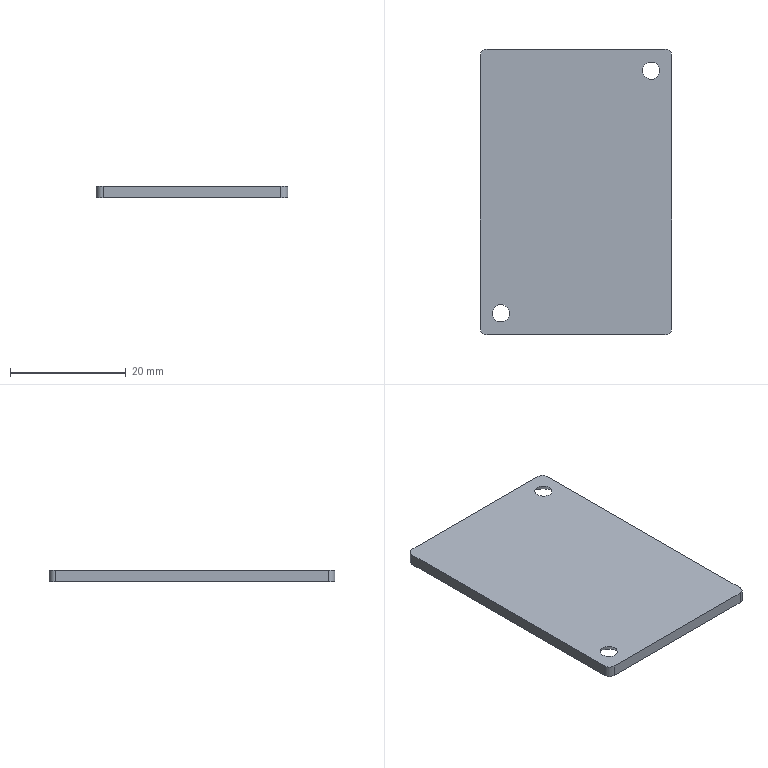Part | STEP file | 4V430C_15_Valve_Board | 1 solid | 14 faces | box 33.2 x 49.5 x 2 mm | volume 3202 mm3 | plane 6 | cone 4 | cylinder 4 | commonest cylinder face diameters 2.4 x4
STEP:
#1=CARTESIAN_POINT('',(0.,0.,0.));
#2=DIRECTION('',(0.,0.,1.));
#3=DIRECTION('',(1.,0.,0.));
#4=AXIS2_PLACEMENT_3D('',#1,#2,#3);
#5=CARTESIAN_POINT('',(-14.5,-21.,0.));
#6=VERTEX_POINT('',#5);
#7=CARTESIAN_POINT('',(-16.5,-21.,-2.));
#8=VERTEX_POINT('',#7);
#9=CARTESIAN_POINT('',(-14.5,-21.,0.));
#10=DIRECTION('',(-0.7071,0.,-0.7071));
#11=VECTOR('',#10,1.);
#12=LINE('',#9,#11);
#13=CARTESIAN_POINT('',(-13.,-21.,0.));
#14=DIRECTION('',(0.,0.,-1.));
#15=DIRECTION('',(-1.,0.,0.));
#16=AXIS2_PLACEMENT_3D('',#13,#14,#15);
#17=CONICAL_SURFACE('',#16,1.5,0.7854);
#18=CARTESIAN_POINT('',(6.283,0.));
#19=DIRECTION('',(0.,1.));
#20=VECTOR('',#19,1.);
#21=LINE('',#18,#20);
#22=(GEOMETRIC_REPRESENTATION_CONTEXT(2)PARAMETRIC_REPRESENTATION_CONTEXT()REPRESENTATION_CONTEXT('',''));
#23=DEFINITIONAL_REPRESENTATION('',(#21),#22);
#24=PCURVE('',#17,#23);
#25=CARTESIAN_POINT('',(-13.,-21.,0.));
#26=DIRECTION('',(0.,0.,-1.));
#27=DIRECTION('',(-1.,0.,0.));
#28=AXIS2_PLACEMENT_3D('',#25,#26,#27);
#29=CONICAL_SURFACE('',#28,1.5,0.7854);
#30=CARTESIAN_POINT('',(0.,0.));
#31=DIRECTION('',(0.,1.));
#32=VECTOR('',#31,1.);
#33=LINE('',#30,#32);
#34=(GEOMETRIC_REPRESENTATION_CONTEXT(2)PARAMETRIC_REPRESENTATION_CONTEXT()REPRESENTATION_CONTEXT('',''));
#35=DEFINITIONAL_REPRESENTATION('',(#33),#34);
#36=PCURVE('',#29,#35);
#37=SURFACE_CURVE('',#12,(#24,#36),.PCURVE_S1.);
#38=EDGE_CURVE('',#6,#8,#37,.T.);
#39=ORIENTED_EDGE('',*,*,#38,.T.);
#40=CARTESIAN_POINT('',(-9.5,-21.,-2.));
#41=VERTEX_POINT('',#40);
#42=CARTESIAN_POINT('',(-13.,-21.,-2.));
#43=DIRECTION('',(0.,0.,-1.));
#44=DIRECTION('',(-1.,0.,0.));
#45=AXIS2_PLACEMENT_3D('',#42,#43,#44);
#46=CIRCLE('',#45,3.5);
#47=CARTESIAN_POINT('',(0.,2.));
#48=DIRECTION('',(1.,0.));
#49=VECTOR('',#48,1.);
#50=LINE('',#47,#49);
#51=(GEOMETRIC_REPRESENTATION_CONTEXT(2)PARAMETRIC_REPRESENTATION_CONTEXT()REPRESENTATION_CONTEXT('',''));
#52=DEFINITIONAL_REPRESENTATION('',(#50),#51);
#53=PCURVE('',#17,#52);
#54=CARTESIAN_POINT('',(-15.4,-23.55,-2.));
#55=DIRECTION('',(0.,0.,1.));
#56=DIRECTION('',(1.,0.,0.));
#57=AXIS2_PLACEMENT_3D('',#54,#55,#56);
#58=PLANE('',#57);
#59=CARTESIAN_POINT('',(-1.1,2.55));
#60=CARTESIAN_POINT('',(-1.1,8.612));
#61=CARTESIAN_POINT('',(4.15,5.581));
#62=CARTESIAN_POINT('',(9.4,2.55));
#63=CARTESIAN_POINT('',(4.15,-0.4811));
#64=CARTESIAN_POINT('',(-1.1,-3.512));
#65=CARTESIAN_POINT('',(-1.1,2.55));
#66=(BOUNDED_CURVE()B_SPLINE_CURVE(2,(#59,#60,#61,#62,#63,#64,#65),.UNSPECIFIED.,.T.,.F.)B_SPLINE_CURVE_WITH_KNOTS((1,2,2,2,2,1),(-2.094,0.,2.094,4.189,6.283,8.378),.UNSPECIFIED.)CURVE()GEOMETRIC_REPRESENTATION_ITEM()RATIONAL_B_SPLINE_CURVE((1.,0.5,1.,0.5,1.,0.5,1.))REPRESENTATION_ITEM(''));
#67=(GEOMETRIC_REPRESENTATION_CONTEXT(2)PARAMETRIC_REPRESENTATION_CONTEXT()REPRESENTATION_CONTEXT('',''));
#68=DEFINITIONAL_REPRESENTATION('',(#66),#67);
#69=PCURVE('',#58,#68);
#70=SURFACE_CURVE('',#46,(#53,#69),.PCURVE_S1.);
#71=EDGE_CURVE('',#41,#8,#70,.T.);
#72=ORIENTED_EDGE('',*,*,#71,.F.);
#73=CARTESIAN_POINT('',(-11.5,-21.,0.));
#74=VERTEX_POINT('',#73);
#75=CARTESIAN_POINT('',(-11.5,-21.,0.));
#76=DIRECTION('',(0.7071,0.,-0.7071));
#77=VECTOR('',#76,1.);
#78=LINE('',#75,#77);
#79=CARTESIAN_POINT('',(3.142,0.));
#80=DIRECTION('',(0.,1.));
#81=VECTOR('',#80,1.);
#82=LINE('',#79,#81);
#83=(GEOMETRIC_REPRESENTATION_CONTEXT(2)PARAMETRIC_REPRESENTATION_CONTEXT()REPRESENTATION_CONTEXT('',''));
#84=DEFINITIONAL_REPRESENTATION('',(#82),#83);
#85=PCURVE('',#17,#84);
#86=CARTESIAN_POINT('',(3.142,0.));
#87=DIRECTION('',(0.,1.));
#88=VECTOR('',#87,1.);
#89=LINE('',#86,#88);
#90=(GEOMETRIC_REPRESENTATION_CONTEXT(2)PARAMETRIC_REPRESENTATION_CONTEXT()REPRESENTATION_CONTEXT('',''));
#91=DEFINITIONAL_REPRESENTATION('',(#89),#90);
#92=PCURVE('',#29,#91);
#93=SURFACE_CURVE('',#78,(#85,#92),.PCURVE_S1.);
#94=EDGE_CURVE('',#74,#41,#93,.T.);
#95=ORIENTED_EDGE('',*,*,#94,.F.);
#96=CARTESIAN_POINT('',(-13.,-21.,0.));
#97=DIRECTION('',(0.,0.,-1.));
#98=DIRECTION('',(-1.,0.,0.));
#99=AXIS2_PLACEMENT_3D('',#96,#97,#98);
#100=CIRCLE('',#99,1.5);
#101=CARTESIAN_POINT('',(0.,0.));
#102=DIRECTION('',(1.,0.));
#103=VECTOR('',#102,1.);
#104=LINE('',#101,#103);
#105=(GEOMETRIC_REPRESENTATION_CONTEXT(2)PARAMETRIC_REPRESENTATION_CONTEXT()REPRESENTATION_CONTEXT('',''));
#106=DEFINITIONAL_REPRESENTATION('',(#104),#105);
#107=PCURVE('',#17,#106);
#108=CARTESIAN_POINT('',(-15.4,-23.55,0.));
#109=DIRECTION('',(0.,0.,1.));
#110=DIRECTION('',(1.,0.,0.));
#111=AXIS2_PLACEMENT_3D('',#108,#109,#110);
#112=PLANE('',#111);
#113=CARTESIAN_POINT('',(0.9,2.55));
#114=CARTESIAN_POINT('',(0.9,5.148));
#115=CARTESIAN_POINT('',(3.15,3.849));
#116=CARTESIAN_POINT('',(5.4,2.55));
#117=CARTESIAN_POINT('',(3.15,1.251));
#118=CARTESIAN_POINT('',(0.9,-0.04808));
#119=CARTESIAN_POINT('',(0.9,2.55));
#120=(BOUNDED_CURVE()B_SPLINE_CURVE(2,(#113,#114,#115,#116,#117,#118,#119),.UNSPECIFIED.,.T.,.F.)B_SPLINE_CURVE_WITH_KNOTS((1,2,2,2,2,1),(-2.094,0.,2.094,4.189,6.283,8.378),.UNSPECIFIED.)CURVE()GEOMETRIC_REPRESENTATION_ITEM()RATIONAL_B_SPLINE_CURVE((1.,0.5,1.,0.5,1.,0.5,1.))REPRESENTATION_ITEM(''));
#121=(GEOMETRIC_REPRESENTATION_CONTEXT(2)PARAMETRIC_REPRESENTATION_CONTEXT()REPRESENTATION_CONTEXT('',''));
#122=DEFINITIONAL_REPRESENTATION('',(#120),#121);
#123=PCURVE('',#112,#122);
#124=SURFACE_CURVE('',#100,(#107,#123),.PCURVE_S1.);
#125=EDGE_CURVE('',#74,#6,#124,.T.);
#126=ORIENTED_EDGE('',*,*,#125,.T.);
#127=EDGE_LOOP('',(#39,#72,#95,#126));
#128=FACE_BOUND('',#127,.F.);
#129=ADVANCED_FACE('',(#128),#17,.F.);
#130=CARTESIAN_POINT('',(11.5,21.,0.));
#131=VERTEX_POINT('',#130);
#132=CARTESIAN_POINT('',(9.5,21.,-2.));
#133=VERTEX_POINT('',#132);
#134=CARTESIAN_POINT('',(9.5,21.,-2.));
#135=DIRECTION('',(-0.7071,0.,-0.7071));
#136=VECTOR('',#135,1.);
#137=LINE('',#134,#136);
#138=CARTESIAN_POINT('',(13.,21.,-2.));
#139=DIRECTION('',(0.,0.,-1.));
#140=DIRECTION('',(-1.,0.,0.));
#141=AXIS2_PLACEMENT_3D('',#138,#139,#140);
#142=CONICAL_SURFACE('',#141,3.5,0.7854);
#143=CARTESIAN_POINT('',(6.283,0.));
#144=DIRECTION('',(0.,1.));
#145=VECTOR('',#144,1.);
#146=LINE('',#143,#145);
#147=(GEOMETRIC_REPRESENTATION_CONTEXT(2)PARAMETRIC_REPRESENTATION_CONTEXT()REPRESENTATION_CONTEXT('',''));
#148=DEFINITIONAL_REPRESENTATION('',(#146),#147);
#149=PCURVE('',#142,#148);
#150=CARTESIAN_POINT('',(13.,21.,-2.));
#151=DIRECTION('',(0.,0.,-1.));
#152=DIRECTION('',(-1.,0.,0.));
#153=AXIS2_PLACEMENT_3D('',#150,#151,#152);
#154=CONICAL_SURFACE('',#153,3.5,0.7854);
#155=CARTESIAN_POINT('',(0.,0.));
#156=DIRECTION('',(0.,1.));
#157=VECTOR('',#156,1.);
#158=LINE('',#155,#157);
#159=(GEOMETRIC_REPRESENTATION_CONTEXT(2)PARAMETRIC_REPRESENTATION_CONTEXT()REPRESENTATION_CONTEXT('',''));
#160=DEFINITIONAL_REPRESENTATION('',(#158),#159);
#161=PCURVE('',#154,#160);
#162=SURFACE_CURVE('',#137,(#149,#161),.PCURVE_S1.);
#163=EDGE_CURVE('',#131,#133,#162,.T.);
#164=ORIENTED_EDGE('',*,*,#163,.T.);
#165=CARTESIAN_POINT('',(16.5,21.,-2.));
#166=VERTEX_POINT('',#165);
#167=CARTESIAN_POINT('',(13.,21.,-2.));
#168=DIRECTION('',(0.,0.,1.));
#169=DIRECTION('',(1.,0.,0.));
#170=AXIS2_PLACEMENT_3D('',#167,#168,#169);
#171=CIRCLE('',#170,3.5);
#172=CARTESIAN_POINT('',(9.425,0.));
#173=DIRECTION('',(-1.,0.));
#174=VECTOR('',#173,1.);
#175=LINE('',#172,#174);
#176=(GEOMETRIC_REPRESENTATION_CONTEXT(2)PARAMETRIC_REPRESENTATION_CONTEXT()REPRESENTATION_CONTEXT('',''));
#177=DEFINITIONAL_REPRESENTATION('',(#175),#176);
#178=PCURVE('',#142,#177);
#179=CARTESIAN_POINT('',(28.4,44.55));
#180=DIRECTION('',(1.,0.));
#181=AXIS2_PLACEMENT_2D('',#179,#180);
#182=CIRCLE('',#181,3.5);
#183=(GEOMETRIC_REPRESENTATION_CONTEXT(2)PARAMETRIC_REPRESENTATION_CONTEXT()REPRESENTATION_CONTEXT('',''));
#184=DEFINITIONAL_REPRESENTATION('',(#182),#183);
#185=PCURVE('',#58,#184);
#186=SURFACE_CURVE('',#171,(#178,#185),.PCURVE_S1.);
#187=EDGE_CURVE('',#133,#166,#186,.T.);
#188=ORIENTED_EDGE('',*,*,#187,.T.);
#189=CARTESIAN_POINT('',(14.5,21.,0.));
#190=VERTEX_POINT('',#189);
#191=CARTESIAN_POINT('',(16.5,21.,-2.));
#192=DIRECTION('',(0.7071,0.,-0.7071));
#193=VECTOR('',#192,1.);
#194=LINE('',#191,#193);
#195=CARTESIAN_POINT('',(3.142,0.));
#196=DIRECTION('',(0.,1.));
#197=VECTOR('',#196,1.);
#198=LINE('',#195,#197);
#199=(GEOMETRIC_REPRESENTATION_CONTEXT(2)PARAMETRIC_REPRESENTATION_CONTEXT()REPRESENTATION_CONTEXT('',''));
#200=DEFINITIONAL_REPRESENTATION('',(#198),#199);
#201=PCURVE('',#142,#200);
#202=CARTESIAN_POINT('',(3.142,0.));
#203=DIRECTION('',(0.,1.));
#204=VECTOR('',#203,1.);
#205=LINE('',#202,#204);
#206=(GEOMETRIC_REPRESENTATION_CONTEXT(2)PARAMETRIC_REPRESENTATION_CONTEXT()REPRESENTATION_CONTEXT('',''));
#207=DEFINITIONAL_REPRESENTATION('',(#205),#206);
#208=PCURVE('',#154,#207);
#209=SURFACE_CURVE('',#194,(#201,#208),.PCURVE_S1.);
#210=EDGE_CURVE('',#190,#166,#209,.T.);
#211=ORIENTED_EDGE('',*,*,#210,.F.);
#212=CARTESIAN_POINT('',(13.,21.,0.));
#213=DIRECTION('',(0.,0.,1.));
#214=DIRECTION('',(1.,0.,0.));
#215=AXIS2_PLACEMENT_3D('',#212,#213,#214);
#216=CIRCLE('',#215,1.5);
#217=CARTESIAN_POINT('',(9.425,-2.));
#218=DIRECTION('',(-1.,0.));
#219=VECTOR('',#218,1.);
#220=LINE('',#217,#219);
#221=(GEOMETRIC_REPRESENTATION_CONTEXT(2)PARAMETRIC_REPRESENTATION_CONTEXT()REPRESENTATION_CONTEXT('',''));
#222=DEFINITIONAL_REPRESENTATION('',(#220),#221);
#223=PCURVE('',#142,#222);
#224=CARTESIAN_POINT('',(28.4,44.55));
#225=DIRECTION('',(1.,0.));
#226=AXIS2_PLACEMENT_2D('',#224,#225);
#227=CIRCLE('',#226,1.5);
#228=(GEOMETRIC_REPRESENTATION_CONTEXT(2)PARAMETRIC_REPRESENTATION_CONTEXT()REPRESENTATION_CONTEXT('',''));
#229=DEFINITIONAL_REPRESENTATION('',(#227),#228);
#230=PCURVE('',#112,#229);
#231=SURFACE_CURVE('',#216,(#223,#230),.PCURVE_S1.);
#232=EDGE_CURVE('',#131,#190,#231,.T.);
#233=ORIENTED_EDGE('',*,*,#232,.F.);
#234=EDGE_LOOP('',(#164,#188,#211,#233));
#235=FACE_BOUND('',#234,.F.);
#236=ADVANCED_FACE('',(#235),#142,.F.);
#237=ORIENTED_EDGE('',*,*,#187,.T.);
#238=CARTESIAN_POINT('',(13.,21.,-2.));
#239=DIRECTION('',(0.,0.,1.));
#240=DIRECTION('',(1.,0.,0.));
#241=AXIS2_PLACEMENT_3D('',#238,#239,#240);
#242=CIRCLE('',#241,3.5);
#243=CARTESIAN_POINT('',(28.4,44.55));
#244=DIRECTION('',(1.,0.));
#245=AXIS2_PLACEMENT_2D('',#243,#244);
#246=CIRCLE('',#245,3.5);
#247=(GEOMETRIC_REPRESENTATION_CONTEXT(2)PARAMETRIC_REPRESENTATION_CONTEXT()REPRESENTATION_CONTEXT('',''));
#248=DEFINITIONAL_REPRESENTATION('',(#246),#247);
#249=PCURVE('',#58,#248);
#250=CARTESIAN_POINT('',(3.142,0.));
#251=DIRECTION('',(-1.,0.));
#252=VECTOR('',#251,1.);
#253=LINE('',#250,#252);
#254=(GEOMETRIC_REPRESENTATION_CONTEXT(2)PARAMETRIC_REPRESENTATION_CONTEXT()REPRESENTATION_CONTEXT('',''));
#255=DEFINITIONAL_REPRESENTATION('',(#253),#254);
#256=PCURVE('',#154,#255);
#257=SURFACE_CURVE('',#242,(#249,#256),.PCURVE_S1.);
#258=EDGE_CURVE('',#166,#133,#257,.T.);
#259=ORIENTED_EDGE('',*,*,#258,.T.);
#260=EDGE_LOOP('',(#237,#259));
#261=FACE_BOUND('',#260,.T.);
#262=CARTESIAN_POINT('',(-16.6,-23.55,-2.));
#263=VERTEX_POINT('',#262);
#264=CARTESIAN_POINT('',(-15.4,-24.75,-2.));
#265=VERTEX_POINT('',#264);
#266=CARTESIAN_POINT('',(-15.4,-23.55,-2.));
#267=DIRECTION('',(0.,0.,1.));
#268=DIRECTION('',(1.,0.,0.));
#269=AXIS2_PLACEMENT_3D('',#266,#267,#268);
#270=CIRCLE('',#269,1.2);
#271=CARTESIAN_POINT('',(0.,0.));
#272=DIRECTION('',(1.,0.));
#273=AXIS2_PLACEMENT_2D('',#271,#272);
#274=CIRCLE('',#273,1.2);
#275=(GEOMETRIC_REPRESENTATION_CONTEXT(2)PARAMETRIC_REPRESENTATION_CONTEXT()REPRESENTATION_CONTEXT('',''));
#276=DEFINITIONAL_REPRESENTATION('',(#274),#275);
#277=PCURVE('',#58,#276);
#278=CARTESIAN_POINT('',(-15.4,-23.55,-2.));
#279=DIRECTION('',(0.,0.,1.));
#280=DIRECTION('',(1.,0.,0.));
#281=AXIS2_PLACEMENT_3D('',#278,#279,#280);
#282=CYLINDRICAL_SURFACE('',#281,1.2);
#283=CARTESIAN_POINT('',(0.,0.));
#284=DIRECTION('',(1.,0.));
#285=VECTOR('',#284,1.);
#286=LINE('',#283,#285);
#287=(GEOMETRIC_REPRESENTATION_CONTEXT(2)PARAMETRIC_REPRESENTATION_CONTEXT()REPRESENTATION_CONTEXT('',''));
#288=DEFINITIONAL_REPRESENTATION('',(#286),#287);
#289=PCURVE('',#282,#288);
#290=SURFACE_CURVE('',#270,(#277,#289),.PCURVE_S1.);
#291=EDGE_CURVE('',#263,#265,#290,.T.);
#292=ORIENTED_EDGE('',*,*,#291,.F.);
#293=CARTESIAN_POINT('',(-16.6,23.55,-2.));
#294=VERTEX_POINT('',#293);
#295=CARTESIAN_POINT('',(-16.6,23.55,-2.));
#296=DIRECTION('',(0.,-1.,0.));
#297=VECTOR('',#296,1.);
#298=LINE('',#295,#297);
#299=CARTESIAN_POINT('',(-1.2,47.1));
#300=DIRECTION('',(0.,-1.));
#301=VECTOR('',#300,1.);
#302=LINE('',#299,#301);
#303=(GEOMETRIC_REPRESENTATION_CONTEXT(2)PARAMETRIC_REPRESENTATION_CONTEXT()REPRESENTATION_CONTEXT('',''));
#304=DEFINITIONAL_REPRESENTATION('',(#302),#303);
#305=PCURVE('',#58,#304);
#306=CARTESIAN_POINT('',(-16.6,23.55,-2.));
#307=DIRECTION('',(-1.,0.,0.));
#308=DIRECTION('',(0.,0.,1.));
#309=AXIS2_PLACEMENT_3D('',#306,#307,#308);
#310=PLANE('',#309);
#311=CARTESIAN_POINT('',(0.,0.));
#312=DIRECTION('',(0.,-1.));
#313=VECTOR('',#312,1.);
#314=LINE('',#311,#313);
#315=(GEOMETRIC_REPRESENTATION_CONTEXT(2)PARAMETRIC_REPRESENTATION_CONTEXT()REPRESENTATION_CONTEXT('',''));
#316=DEFINITIONAL_REPRESENTATION('',(#314),#315);
#317=PCURVE('',#310,#316);
#318=SURFACE_CURVE('',#298,(#305,#317),.PCURVE_S1.);
#319=EDGE_CURVE('',#294,#263,#318,.T.);
#320=ORIENTED_EDGE('',*,*,#319,.F.);
#321=CARTESIAN_POINT('',(-15.4,24.75,-2.));
#322=VERTEX_POINT('',#321);
#323=CARTESIAN_POINT('',(-15.4,23.55,-2.));
#324=DIRECTION('',(0.,0.,1.));
#325=DIRECTION('',(1.,0.,0.));
#326=AXIS2_PLACEMENT_3D('',#323,#324,#325);
#327=CIRCLE('',#326,1.2);
#328=CARTESIAN_POINT('',(0.,47.1));
#329=DIRECTION('',(1.,0.));
#330=AXIS2_PLACEMENT_2D('',#328,#329);
#331=CIRCLE('',#330,1.2);
#332=(GEOMETRIC_REPRESENTATION_CONTEXT(2)PARAMETRIC_REPRESENTATION_CONTEXT()REPRESENTATION_CONTEXT('',''));
#333=DEFINITIONAL_REPRESENTATION('',(#331),#332);
#334=PCURVE('',#58,#333);
#335=CARTESIAN_POINT('',(-15.4,23.55,-2.));
#336=DIRECTION('',(0.,0.,1.));
#337=DIRECTION('',(1.,0.,0.));
#338=AXIS2_PLACEMENT_3D('',#335,#336,#337);
#339=CYLINDRICAL_SURFACE('',#338,1.2);
#340=CARTESIAN_POINT('',(0.,0.));
#341=DIRECTION('',(1.,0.));
#342=VECTOR('',#341,1.);
#343=LINE('',#340,#342);
#344=(GEOMETRIC_REPRESENTATION_CONTEXT(2)PARAMETRIC_REPRESENTATION_CONTEXT()REPRESENTATION_CONTEXT('',''));
#345=DEFINITIONAL_REPRESENTATION('',(#343),#344);
#346=PCURVE('',#339,#345);
#347=SURFACE_CURVE('',#327,(#334,#346),.PCURVE_S1.);
#348=EDGE_CURVE('',#322,#294,#347,.T.);
#349=ORIENTED_EDGE('',*,*,#348,.F.);
#350=CARTESIAN_POINT('',(15.4,24.75,-2.));
#351=VERTEX_POINT('',#350);
#352=CARTESIAN_POINT('',(15.4,24.75,-2.));
#353=DIRECTION('',(-1.,0.,0.));
#354=VECTOR('',#353,1.);
#355=LINE('',#352,#354);
#356=CARTESIAN_POINT('',(30.8,48.3));
#357=DIRECTION('',(-1.,0.));
#358=VECTOR('',#357,1.);
#359=LINE('',#356,#358);
#360=(GEOMETRIC_REPRESENTATION_CONTEXT(2)PARAMETRIC_REPRESENTATION_CONTEXT()REPRESENTATION_CONTEXT('',''));
#361=DEFINITIONAL_REPRESENTATION('',(#359),#360);
#362=PCURVE('',#58,#361);
#363=CARTESIAN_POINT('',(15.4,24.75,-2.));
#364=DIRECTION('',(0.,1.,0.));
#365=DIRECTION('',(0.,0.,1.));
#366=AXIS2_PLACEMENT_3D('',#363,#364,#365);
#367=PLANE('',#366);
#368=CARTESIAN_POINT('',(0.,0.));
#369=DIRECTION('',(0.,-1.));
#370=VECTOR('',#369,1.);
#371=LINE('',#368,#370);
#372=(GEOMETRIC_REPRESENTATION_CONTEXT(2)PARAMETRIC_REPRESENTATION_CONTEXT()REPRESENTATION_CONTEXT('',''));
#373=DEFINITIONAL_REPRESENTATION('',(#371),#372);
#374=PCURVE('',#367,#373);
#375=SURFACE_CURVE('',#355,(#362,#374),.PCURVE_S1.);
#376=EDGE_CURVE('',#351,#322,#375,.T.);
#377=ORIENTED_EDGE('',*,*,#376,.F.);
#378=CARTESIAN_POINT('',(16.6,23.55,-2.));
#379=VERTEX_POINT('',#378);
#380=CARTESIAN_POINT('',(15.4,23.55,-2.));
#381=DIRECTION('',(0.,0.,1.));
#382=DIRECTION('',(1.,0.,0.));
#383=AXIS2_PLACEMENT_3D('',#380,#381,#382);
#384=CIRCLE('',#383,1.2);
#385=CARTESIAN_POINT('',(30.8,47.1));
#386=DIRECTION('',(1.,0.));
#387=AXIS2_PLACEMENT_2D('',#385,#386);
#388=CIRCLE('',#387,1.2);
#389=(GEOMETRIC_REPRESENTATION_CONTEXT(2)PARAMETRIC_REPRESENTATION_CONTEXT()REPRESENTATION_CONTEXT('',''));
#390=DEFINITIONAL_REPRESENTATION('',(#388),#389);
#391=PCURVE('',#58,#390);
#392=CARTESIAN_POINT('',(15.4,23.55,-2.));
#393=DIRECTION('',(0.,0.,1.));
#394=DIRECTION('',(1.,0.,0.));
#395=AXIS2_PLACEMENT_3D('',#392,#393,#394);
#396=CYLINDRICAL_SURFACE('',#395,1.2);
#397=CARTESIAN_POINT('',(0.,0.));
#398=DIRECTION('',(1.,0.));
#399=VECTOR('',#398,1.);
#400=LINE('',#397,#399);
#401=(GEOMETRIC_REPRESENTATION_CONTEXT(2)PARAMETRIC_REPRESENTATION_CONTEXT()REPRESENTATION_CONTEXT('',''));
#402=DEFINITIONAL_REPRESENTATION('',(#400),#401);
#403=PCURVE('',#396,#402);
#404=SURFACE_CURVE('',#384,(#391,#403),.PCURVE_S1.);
#405=EDGE_CURVE('',#379,#351,#404,.T.);
#406=ORIENTED_EDGE('',*,*,#405,.F.);
#407=CARTESIAN_POINT('',(16.6,-23.55,-2.));
#408=VERTEX_POINT('',#407);
#409=CARTESIAN_POINT('',(16.6,-23.55,-2.));
#410=DIRECTION('',(0.,1.,0.));
#411=VECTOR('',#410,1.);
#412=LINE('',#409,#411);
#413=CARTESIAN_POINT('',(32.,0.));
#414=DIRECTION('',(0.,1.));
#415=VECTOR('',#414,1.);
#416=LINE('',#413,#415);
#417=(GEOMETRIC_REPRESENTATION_CONTEXT(2)PARAMETRIC_REPRESENTATION_CONTEXT()REPRESENTATION_CONTEXT('',''));
#418=DEFINITIONAL_REPRESENTATION('',(#416),#417);
#419=PCURVE('',#58,#418);
#420=CARTESIAN_POINT('',(16.6,-23.55,-2.));
#421=DIRECTION('',(1.,0.,0.));
#422=DIRECTION('',(0.,0.,-1.));
#423=AXIS2_PLACEMENT_3D('',#420,#421,#422);
#424=PLANE('',#423);
#425=CARTESIAN_POINT('',(0.,0.));
#426=DIRECTION('',(0.,1.));
#427=VECTOR('',#426,1.);
#428=LINE('',#425,#427);
#429=(GEOMETRIC_REPRESENTATION_CONTEXT(2)PARAMETRIC_REPRESENTATION_CONTEXT()REPRESENTATION_CONTEXT('',''));
#430=DEFINITIONAL_REPRESENTATION('',(#428),#429);
#431=PCURVE('',#424,#430);
#432=SURFACE_CURVE('',#412,(#419,#431),.PCURVE_S1.);
#433=EDGE_CURVE('',#408,#379,#432,.T.);
#434=ORIENTED_EDGE('',*,*,#433,.F.);
#435=CARTESIAN_POINT('',(15.4,-24.75,-2.));
#436=VERTEX_POINT('',#435);
#437=CARTESIAN_POINT('',(15.4,-23.55,-2.));
#438=DIRECTION('',(0.,0.,1.));
#439=DIRECTION('',(1.,0.,0.));
#440=AXIS2_PLACEMENT_3D('',#437,#438,#439);
#441=CIRCLE('',#440,1.2);
#442=CARTESIAN_POINT('',(30.8,0.));
#443=DIRECTION('',(1.,0.));
#444=AXIS2_PLACEMENT_2D('',#442,#443);
#445=CIRCLE('',#444,1.2);
#446=(GEOMETRIC_REPRESENTATION_CONTEXT(2)PARAMETRIC_REPRESENTATION_CONTEXT()REPRESENTATION_CONTEXT('',''));
#447=DEFINITIONAL_REPRESENTATION('',(#445),#446);
#448=PCURVE('',#58,#447);
#449=CARTESIAN_POINT('',(15.4,-23.55,-2.));
#450=DIRECTION('',(0.,0.,1.));
#451=DIRECTION('',(1.,0.,0.));
#452=AXIS2_PLACEMENT_3D('',#449,#450,#451);
#453=CYLINDRICAL_SURFACE('',#452,1.2);
#454=CARTESIAN_POINT('',(0.,0.));
#455=DIRECTION('',(1.,0.));
#456=VECTOR('',#455,1.);
#457=LINE('',#454,#456);
#458=(GEOMETRIC_REPRESENTATION_CONTEXT(2)PARAMETRIC_REPRESENTATION_CONTEXT()REPRESENTATION_CONTEXT('',''));
#459=DEFINITIONAL_REPRESENTATION('',(#457),#458);
#460=PCURVE('',#453,#459);
#461=SURFACE_CURVE('',#441,(#448,#460),.PCURVE_S1.);
#462=EDGE_CURVE('',#436,#408,#461,.T.);
#463=ORIENTED_EDGE('',*,*,#462,.F.);
#464=CARTESIAN_POINT('',(-15.4,-24.75,-2.));
#465=DIRECTION('',(1.,0.,0.));
#466=VECTOR('',#465,1.);
#467=LINE('',#464,#466);
#468=CARTESIAN_POINT('',(0.,-1.2));
#469=DIRECTION('',(1.,0.));
#470=VECTOR('',#469,1.);
#471=LINE('',#468,#470);
#472=(GEOMETRIC_REPRESENTATION_CONTEXT(2)PARAMETRIC_REPRESENTATION_CONTEXT()REPRESENTATION_CONTEXT('',''));
#473=DEFINITIONAL_REPRESENTATION('',(#471),#472);
#474=PCURVE('',#58,#473);
#475=CARTESIAN_POINT('',(-15.4,-24.75,-2.));
#476=DIRECTION('',(0.,-1.,0.));
#477=DIRECTION('',(0.,0.,-1.));
#478=AXIS2_PLACEMENT_3D('',#475,#476,#477);
#479=PLANE('',#478);
#480=CARTESIAN_POINT('',(0.,0.));
#481=DIRECTION('',(0.,1.));
#482=VECTOR('',#481,1.);
#483=LINE('',#480,#482);
#484=(GEOMETRIC_REPRESENTATION_CONTEXT(2)PARAMETRIC_REPRESENTATION_CONTEXT()REPRESENTATION_CONTEXT('',''));
#485=DEFINITIONAL_REPRESENTATION('',(#483),#484);
#486=PCURVE('',#479,#485);
#487=SURFACE_CURVE('',#467,(#474,#486),.PCURVE_S1.);
#488=EDGE_CURVE('',#265,#436,#487,.T.);
#489=ORIENTED_EDGE('',*,*,#488,.F.);
#490=EDGE_LOOP('',(#292,#320,#349,#377,#406,#434,#463,#489));
#491=FACE_BOUND('',#490,.T.);
#492=CARTESIAN_POINT('',(-13.,-21.,-2.));
#493=DIRECTION('',(0.,0.,-1.));
#494=DIRECTION('',(-1.,0.,0.));
#495=AXIS2_PLACEMENT_3D('',#492,#493,#494);
#496=CIRCLE('',#495,3.5);
#497=CARTESIAN_POINT('',(-1.1,2.55));
#498=CARTESIAN_POINT('',(-1.1,8.612));
#499=CARTESIAN_POINT('',(4.15,5.581));
#500=CARTESIAN_POINT('',(9.4,2.55));
#501=CARTESIAN_POINT('',(4.15,-0.4811));
#502=CARTESIAN_POINT('',(-1.1,-3.512));
#503=CARTESIAN_POINT('',(-1.1,2.55));
#504=(BOUNDED_CURVE()B_SPLINE_CURVE(2,(#497,#498,#499,#500,#501,#502,#503),.UNSPECIFIED.,.T.,.F.)B_SPLINE_CURVE_WITH_KNOTS((1,2,2,2,2,1),(-2.094,0.,2.094,4.189,6.283,8.378),.UNSPECIFIED.)CURVE()GEOMETRIC_REPRESENTATION_ITEM()RATIONAL_B_SPLINE_CURVE((1.,0.5,1.,0.5,1.,0.5,1.))REPRESENTATION_ITEM(''));
#505=(GEOMETRIC_REPRESENTATION_CONTEXT(2)PARAMETRIC_REPRESENTATION_CONTEXT()REPRESENTATION_CONTEXT('',''));
#506=DEFINITIONAL_REPRESENTATION('',(#504),#505);
#507=PCURVE('',#58,#506);
#508=CARTESIAN_POINT('',(0.,2.));
#509=DIRECTION('',(1.,0.));
#510=VECTOR('',#509,1.);
#511=LINE('',#508,#510);
#512=(GEOMETRIC_REPRESENTATION_CONTEXT(2)PARAMETRIC_REPRESENTATION_CONTEXT()REPRESENTATION_CONTEXT('',''));
#513=DEFINITIONAL_REPRESENTATION('',(#511),#512);
#514=PCURVE('',#29,#513);
#515=SURFACE_CURVE('',#496,(#507,#514),.PCURVE_S1.);
#516=EDGE_CURVE('',#8,#41,#515,.T.);
#517=ORIENTED_EDGE('',*,*,#516,.F.);
#518=ORIENTED_EDGE('',*,*,#71,.F.);
#519=EDGE_LOOP('',(#517,#518));
#520=FACE_BOUND('',#519,.T.);
#521=ADVANCED_FACE('',(#261,#491,#520),#58,.F.);
#522=ORIENTED_EDGE('',*,*,#232,.F.);
#523=CARTESIAN_POINT('',(13.,21.,0.));
#524=DIRECTION('',(0.,0.,1.));
#525=DIRECTION('',(1.,0.,0.));
#526=AXIS2_PLACEMENT_3D('',#523,#524,#525);
#527=CIRCLE('',#526,1.5);
#528=CARTESIAN_POINT('',(28.4,44.55));
#529=DIRECTION('',(1.,0.));
#530=AXIS2_PLACEMENT_2D('',#528,#529);
#531=CIRCLE('',#530,1.5);
#532=(GEOMETRIC_REPRESENTATION_CONTEXT(2)PARAMETRIC_REPRESENTATION_CONTEXT()REPRESENTATION_CONTEXT('',''));
#533=DEFINITIONAL_REPRESENTATION('',(#531),#532);
#534=PCURVE('',#112,#533);
#535=CARTESIAN_POINT('',(3.142,-2.));
#536=DIRECTION('',(-1.,0.));
#537=VECTOR('',#536,1.);
#538=LINE('',#535,#537);
#539=(GEOMETRIC_REPRESENTATION_CONTEXT(2)PARAMETRIC_REPRESENTATION_CONTEXT()REPRESENTATION_CONTEXT('',''));
#540=DEFINITIONAL_REPRESENTATION('',(#538),#539);
#541=PCURVE('',#154,#540);
#542=SURFACE_CURVE('',#527,(#534,#541),.PCURVE_S1.);
#543=EDGE_CURVE('',#190,#131,#542,.T.);
#544=ORIENTED_EDGE('',*,*,#543,.F.);
#545=EDGE_LOOP('',(#522,#544));
#546=FACE_BOUND('',#545,.T.);
#547=CARTESIAN_POINT('',(-16.6,-23.55,0.));
#548=VERTEX_POINT('',#547);
#549=CARTESIAN_POINT('',(-15.4,-24.75,0.));
#550=VERTEX_POINT('',#549);
#551=CARTESIAN_POINT('',(-15.4,-23.55,0.));
#552=DIRECTION('',(0.,0.,1.));
#553=DIRECTION('',(1.,0.,0.));
#554=AXIS2_PLACEMENT_3D('',#551,#552,#553);
#555=CIRCLE('',#554,1.2);
#556=CARTESIAN_POINT('',(0.,0.));
#557=DIRECTION('',(1.,0.));
#558=AXIS2_PLACEMENT_2D('',#556,#557);
#559=CIRCLE('',#558,1.2);
#560=(GEOMETRIC_REPRESENTATION_CONTEXT(2)PARAMETRIC_REPRESENTATION_CONTEXT()REPRESENTATION_CONTEXT('',''));
#561=DEFINITIONAL_REPRESENTATION('',(#559),#560);
#562=PCURVE('',#112,#561);
#563=CARTESIAN_POINT('',(0.,2.));
#564=DIRECTION('',(1.,0.));
#565=VECTOR('',#564,1.);
#566=LINE('',#563,#565);
#567=(GEOMETRIC_REPRESENTATION_CONTEXT(2)PARAMETRIC_REPRESENTATION_CONTEXT()REPRESENTATION_CONTEXT('',''));
#568=DEFINITIONAL_REPRESENTATION('',(#566),#567);
#569=PCURVE('',#282,#568);
#570=SURFACE_CURVE('',#555,(#562,#569),.PCURVE_S1.);
#571=EDGE_CURVE('',#548,#550,#570,.T.);
#572=ORIENTED_EDGE('',*,*,#571,.T.);
#573=CARTESIAN_POINT('',(15.4,-24.75,0.));
#574=VERTEX_POINT('',#573);
#575=CARTESIAN_POINT('',(-15.4,-24.75,0.));
#576=DIRECTION('',(1.,0.,0.));
#577=VECTOR('',#576,1.);
#578=LINE('',#575,#577);
#579=CARTESIAN_POINT('',(0.,-1.2));
#580=DIRECTION('',(1.,0.));
#581=VECTOR('',#580,1.);
#582=LINE('',#579,#581);
#583=(GEOMETRIC_REPRESENTATION_CONTEXT(2)PARAMETRIC_REPRESENTATION_CONTEXT()REPRESENTATION_CONTEXT('',''));
#584=DEFINITIONAL_REPRESENTATION('',(#582),#583);
#585=PCURVE('',#112,#584);
#586=CARTESIAN_POINT('',(-2.,0.));
#587=DIRECTION('',(0.,1.));
#588=VECTOR('',#587,1.);
#589=LINE('',#586,#588);
#590=(GEOMETRIC_REPRESENTATION_CONTEXT(2)PARAMETRIC_REPRESENTATION_CONTEXT()REPRESENTATION_CONTEXT('',''));
#591=DEFINITIONAL_REPRESENTATION('',(#589),#590);
#592=PCURVE('',#479,#591);
#593=SURFACE_CURVE('',#578,(#585,#592),.PCURVE_S1.);
#594=EDGE_CURVE('',#550,#574,#593,.T.);
#595=ORIENTED_EDGE('',*,*,#594,.T.);
#596=CARTESIAN_POINT('',(16.6,-23.55,0.));
#597=VERTEX_POINT('',#596);
#598=CARTESIAN_POINT('',(15.4,-23.55,0.));
#599=DIRECTION('',(0.,0.,1.));
#600=DIRECTION('',(1.,0.,0.));
#601=AXIS2_PLACEMENT_3D('',#598,#599,#600);
#602=CIRCLE('',#601,1.2);
#603=CARTESIAN_POINT('',(30.8,0.));
#604=DIRECTION('',(1.,0.));
#605=AXIS2_PLACEMENT_2D('',#603,#604);
#606=CIRCLE('',#605,1.2);
#607=(GEOMETRIC_REPRESENTATION_CONTEXT(2)PARAMETRIC_REPRESENTATION_CONTEXT()REPRESENTATION_CONTEXT('',''));
#608=DEFINITIONAL_REPRESENTATION('',(#606),#607);
#609=PCURVE('',#112,#608);
#610=CARTESIAN_POINT('',(0.,2.));
#611=DIRECTION('',(1.,0.));
#612=VECTOR('',#611,1.);
#613=LINE('',#610,#612);
#614=(GEOMETRIC_REPRESENTATION_CONTEXT(2)PARAMETRIC_REPRESENTATION_CONTEXT()REPRESENTATION_CONTEXT('',''));
#615=DEFINITIONAL_REPRESENTATION('',(#613),#614);
#616=PCURVE('',#453,#615);
#617=SURFACE_CURVE('',#602,(#609,#616),.PCURVE_S1.);
#618=EDGE_CURVE('',#574,#597,#617,.T.);
#619=ORIENTED_EDGE('',*,*,#618,.T.);
#620=CARTESIAN_POINT('',(16.6,23.55,0.));
#621=VERTEX_POINT('',#620);
#622=CARTESIAN_POINT('',(16.6,-23.55,0.));
#623=DIRECTION('',(0.,1.,0.));
#624=VECTOR('',#623,1.);
#625=LINE('',#622,#624);
#626=CARTESIAN_POINT('',(32.,0.));
#627=DIRECTION('',(0.,1.));
#628=VECTOR('',#627,1.);
#629=LINE('',#626,#628);
#630=(GEOMETRIC_REPRESENTATION_CONTEXT(2)PARAMETRIC_REPRESENTATION_CONTEXT()REPRESENTATION_CONTEXT('',''));
#631=DEFINITIONAL_REPRESENTATION('',(#629),#630);
#632=PCURVE('',#112,#631);
#633=CARTESIAN_POINT('',(-2.,0.));
#634=DIRECTION('',(0.,1.));
#635=VECTOR('',#634,1.);
#636=LINE('',#633,#635);
#637=(GEOMETRIC_REPRESENTATION_CONTEXT(2)PARAMETRIC_REPRESENTATION_CONTEXT()REPRESENTATION_CONTEXT('',''));
#638=DEFINITIONAL_REPRESENTATION('',(#636),#637);
#639=PCURVE('',#424,#638);
#640=SURFACE_CURVE('',#625,(#632,#639),.PCURVE_S1.);
#641=EDGE_CURVE('',#597,#621,#640,.T.);
#642=ORIENTED_EDGE('',*,*,#641,.T.);
#643=CARTESIAN_POINT('',(15.4,24.75,0.));
#644=VERTEX_POINT('',#643);
#645=CARTESIAN_POINT('',(15.4,23.55,0.));
#646=DIRECTION('',(0.,0.,1.));
#647=DIRECTION('',(1.,0.,0.));
#648=AXIS2_PLACEMENT_3D('',#645,#646,#647);
#649=CIRCLE('',#648,1.2);
#650=CARTESIAN_POINT('',(30.8,47.1));
#651=DIRECTION('',(1.,0.));
#652=AXIS2_PLACEMENT_2D('',#650,#651);
#653=CIRCLE('',#652,1.2);
#654=(GEOMETRIC_REPRESENTATION_CONTEXT(2)PARAMETRIC_REPRESENTATION_CONTEXT()REPRESENTATION_CONTEXT('',''));
#655=DEFINITIONAL_REPRESENTATION('',(#653),#654);
#656=PCURVE('',#112,#655);
#657=CARTESIAN_POINT('',(0.,2.));
#658=DIRECTION('',(1.,0.));
#659=VECTOR('',#658,1.);
#660=LINE('',#657,#659);
#661=(GEOMETRIC_REPRESENTATION_CONTEXT(2)PARAMETRIC_REPRESENTATION_CONTEXT()REPRESENTATION_CONTEXT('',''));
#662=DEFINITIONAL_REPRESENTATION('',(#660),#661);
#663=PCURVE('',#396,#662);
#664=SURFACE_CURVE('',#649,(#656,#663),.PCURVE_S1.);
#665=EDGE_CURVE('',#621,#644,#664,.T.);
#666=ORIENTED_EDGE('',*,*,#665,.T.);
#667=CARTESIAN_POINT('',(-15.4,24.75,0.));
#668=VERTEX_POINT('',#667);
#669=CARTESIAN_POINT('',(15.4,24.75,0.));
#670=DIRECTION('',(-1.,0.,0.));
#671=VECTOR('',#670,1.);
#672=LINE('',#669,#671);
#673=CARTESIAN_POINT('',(30.8,48.3));
#674=DIRECTION('',(-1.,0.));
#675=VECTOR('',#674,1.);
#676=LINE('',#673,#675);
#677=(GEOMETRIC_REPRESENTATION_CONTEXT(2)PARAMETRIC_REPRESENTATION_CONTEXT()REPRESENTATION_CONTEXT('',''));
#678=DEFINITIONAL_REPRESENTATION('',(#676),#677);
#679=PCURVE('',#112,#678);
#680=CARTESIAN_POINT('',(2.,0.));
#681=DIRECTION('',(0.,-1.));
#682=VECTOR('',#681,1.);
#683=LINE('',#680,#682);
#684=(GEOMETRIC_REPRESENTATION_CONTEXT(2)PARAMETRIC_REPRESENTATION_CONTEXT()REPRESENTATION_CONTEXT('',''));
#685=DEFINITIONAL_REPRESENTATION('',(#683),#684);
#686=PCURVE('',#367,#685);
#687=SURFACE_CURVE('',#672,(#679,#686),.PCURVE_S1.);
#688=EDGE_CURVE('',#644,#668,#687,.T.);
#689=ORIENTED_EDGE('',*,*,#688,.T.);
#690=CARTESIAN_POINT('',(-16.6,23.55,0.));
#691=VERTEX_POINT('',#690);
#692=CARTESIAN_POINT('',(-15.4,23.55,0.));
#693=DIRECTION('',(0.,0.,1.));
#694=DIRECTION('',(1.,0.,0.));
#695=AXIS2_PLACEMENT_3D('',#692,#693,#694);
#696=CIRCLE('',#695,1.2);
#697=CARTESIAN_POINT('',(0.,47.1));
#698=DIRECTION('',(1.,0.));
#699=AXIS2_PLACEMENT_2D('',#697,#698);
#700=CIRCLE('',#699,1.2);
#701=(GEOMETRIC_REPRESENTATION_CONTEXT(2)PARAMETRIC_REPRESENTATION_CONTEXT()REPRESENTATION_CONTEXT('',''));
#702=DEFINITIONAL_REPRESENTATION('',(#700),#701);
#703=PCURVE('',#112,#702);
#704=CARTESIAN_POINT('',(0.,2.));
#705=DIRECTION('',(1.,0.));
#706=VECTOR('',#705,1.);
#707=LINE('',#704,#706);
#708=(GEOMETRIC_REPRESENTATION_CONTEXT(2)PARAMETRIC_REPRESENTATION_CONTEXT()REPRESENTATION_CONTEXT('',''));
#709=DEFINITIONAL_REPRESENTATION('',(#707),#708);
#710=PCURVE('',#339,#709);
#711=SURFACE_CURVE('',#696,(#703,#710),.PCURVE_S1.);
#712=EDGE_CURVE('',#668,#691,#711,.T.);
#713=ORIENTED_EDGE('',*,*,#712,.T.);
#714=CARTESIAN_POINT('',(-16.6,23.55,0.));
#715=DIRECTION('',(0.,-1.,0.));
#716=VECTOR('',#715,1.);
#717=LINE('',#714,#716);
#718=CARTESIAN_POINT('',(-1.2,47.1));
#719=DIRECTION('',(0.,-1.));
#720=VECTOR('',#719,1.);
#721=LINE('',#718,#720);
#722=(GEOMETRIC_REPRESENTATION_CONTEXT(2)PARAMETRIC_REPRESENTATION_CONTEXT()REPRESENTATION_CONTEXT('',''));
#723=DEFINITIONAL_REPRESENTATION('',(#721),#722);
#724=PCURVE('',#112,#723);
#725=CARTESIAN_POINT('',(2.,0.));
#726=DIRECTION('',(0.,-1.));
#727=VECTOR('',#726,1.);
#728=LINE('',#725,#727);
#729=(GEOMETRIC_REPRESENTATION_CONTEXT(2)PARAMETRIC_REPRESENTATION_CONTEXT()REPRESENTATION_CONTEXT('',''));
#730=DEFINITIONAL_REPRESENTATION('',(#728),#729);
#731=PCURVE('',#310,#730);
#732=SURFACE_CURVE('',#717,(#724,#731),.PCURVE_S1.);
#733=EDGE_CURVE('',#691,#548,#732,.T.);
#734=ORIENTED_EDGE('',*,*,#733,.T.);
#735=EDGE_LOOP('',(#572,#595,#619,#642,#666,#689,#713,#734));
#736=FACE_BOUND('',#735,.T.);
#737=CARTESIAN_POINT('',(-13.,-21.,0.));
#738=DIRECTION('',(0.,0.,-1.));
#739=DIRECTION('',(-1.,0.,0.));
#740=AXIS2_PLACEMENT_3D('',#737,#738,#739);
#741=CIRCLE('',#740,1.5);
#742=CARTESIAN_POINT('',(0.9,2.55));
#743=CARTESIAN_POINT('',(0.9,5.148));
#744=CARTESIAN_POINT('',(3.15,3.849));
#745=CARTESIAN_POINT('',(5.4,2.55));
#746=CARTESIAN_POINT('',(3.15,1.251));
#747=CARTESIAN_POINT('',(0.9,-0.04808));
#748=CARTESIAN_POINT('',(0.9,2.55));
#749=(BOUNDED_CURVE()B_SPLINE_CURVE(2,(#742,#743,#744,#745,#746,#747,#748),.UNSPECIFIED.,.T.,.F.)B_SPLINE_CURVE_WITH_KNOTS((1,2,2,2,2,1),(-2.094,0.,2.094,4.189,6.283,8.378),.UNSPECIFIED.)CURVE()GEOMETRIC_REPRESENTATION_ITEM()RATIONAL_B_SPLINE_CURVE((1.,0.5,1.,0.5,1.,0.5,1.))REPRESENTATION_ITEM(''));
#750=(GEOMETRIC_REPRESENTATION_CONTEXT(2)PARAMETRIC_REPRESENTATION_CONTEXT()REPRESENTATION_CONTEXT('',''));
#751=DEFINITIONAL_REPRESENTATION('',(#749),#750);
#752=PCURVE('',#112,#751);
#753=CARTESIAN_POINT('',(0.,0.));
#754=DIRECTION('',(1.,0.));
#755=VECTOR('',#754,1.);
#756=LINE('',#753,#755);
#757=(GEOMETRIC_REPRESENTATION_CONTEXT(2)PARAMETRIC_REPRESENTATION_CONTEXT()REPRESENTATION_CONTEXT('',''));
#758=DEFINITIONAL_REPRESENTATION('',(#756),#757);
#759=PCURVE('',#29,#758);
#760=SURFACE_CURVE('',#741,(#752,#759),.PCURVE_S1.);
#761=EDGE_CURVE('',#6,#74,#760,.T.);
#762=ORIENTED_EDGE('',*,*,#761,.T.);
#763=ORIENTED_EDGE('',*,*,#125,.T.);
#764=EDGE_LOOP('',(#762,#763));
#765=FACE_BOUND('',#764,.T.);
#766=ADVANCED_FACE('',(#546,#736,#765),#112,.T.);
#767=ORIENTED_EDGE('',*,*,#571,.F.);
#768=CARTESIAN_POINT('',(-16.6,-23.55,-2.));
#769=DIRECTION('',(0.,0.,1.));
#770=VECTOR('',#769,1.);
#771=LINE('',#768,#770);
#772=CARTESIAN_POINT('',(3.142,0.));
#773=DIRECTION('',(0.,1.));
#774=VECTOR('',#773,1.);
#775=LINE('',#772,#774);
#776=(GEOMETRIC_REPRESENTATION_CONTEXT(2)PARAMETRIC_REPRESENTATION_CONTEXT()REPRESENTATION_CONTEXT('',''));
#777=DEFINITIONAL_REPRESENTATION('',(#775),#776);
#778=PCURVE('',#282,#777);
#779=CARTESIAN_POINT('',(0.,-47.1));
#780=DIRECTION('',(1.,0.));
#781=VECTOR('',#780,1.);
#782=LINE('',#779,#781);
#783=(GEOMETRIC_REPRESENTATION_CONTEXT(2)PARAMETRIC_REPRESENTATION_CONTEXT()REPRESENTATION_CONTEXT('',''));
#784=DEFINITIONAL_REPRESENTATION('',(#782),#783);
#785=PCURVE('',#310,#784);
#786=SURFACE_CURVE('',#771,(#778,#785),.PCURVE_S1.);
#787=EDGE_CURVE('',#263,#548,#786,.T.);
#788=ORIENTED_EDGE('',*,*,#787,.F.);
#789=ORIENTED_EDGE('',*,*,#291,.T.);
#790=CARTESIAN_POINT('',(-15.4,-24.75,-2.));
#791=DIRECTION('',(0.,0.,1.));
#792=VECTOR('',#791,1.);
#793=LINE('',#790,#792);
#794=CARTESIAN_POINT('',(4.712,0.));
#795=DIRECTION('',(0.,1.));
#796=VECTOR('',#795,1.);
#797=LINE('',#794,#796);
#798=(GEOMETRIC_REPRESENTATION_CONTEXT(2)PARAMETRIC_REPRESENTATION_CONTEXT()REPRESENTATION_CONTEXT('',''));
#799=DEFINITIONAL_REPRESENTATION('',(#797),#798);
#800=PCURVE('',#282,#799);
#801=CARTESIAN_POINT('',(0.,0.));
#802=DIRECTION('',(-1.,0.));
#803=VECTOR('',#802,1.);
#804=LINE('',#801,#803);
#805=(GEOMETRIC_REPRESENTATION_CONTEXT(2)PARAMETRIC_REPRESENTATION_CONTEXT()REPRESENTATION_CONTEXT('',''));
#806=DEFINITIONAL_REPRESENTATION('',(#804),#805);
#807=PCURVE('',#479,#806);
#808=SURFACE_CURVE('',#793,(#800,#807),.PCURVE_S1.);
#809=EDGE_CURVE('',#265,#550,#808,.T.);
#810=ORIENTED_EDGE('',*,*,#809,.T.);
#811=EDGE_LOOP('',(#767,#788,#789,#810));
#812=FACE_BOUND('',#811,.T.);
#813=ADVANCED_FACE('',(#812),#282,.T.);
#814=ORIENTED_EDGE('',*,*,#733,.F.);
#815=CARTESIAN_POINT('',(-16.6,23.55,-2.));
#816=DIRECTION('',(0.,0.,1.));
#817=VECTOR('',#816,1.);
#818=LINE('',#815,#817);
#819=CARTESIAN_POINT('',(0.,0.));
#820=DIRECTION('',(1.,0.));
#821=VECTOR('',#820,1.);
#822=LINE('',#819,#821);
#823=(GEOMETRIC_REPRESENTATION_CONTEXT(2)PARAMETRIC_REPRESENTATION_CONTEXT()REPRESENTATION_CONTEXT('',''));
#824=DEFINITIONAL_REPRESENTATION('',(#822),#823);
#825=PCURVE('',#310,#824);
#826=CARTESIAN_POINT('',(3.142,0.));
#827=DIRECTION('',(0.,1.));
#828=VECTOR('',#827,1.);
#829=LINE('',#826,#828);
#830=(GEOMETRIC_REPRESENTATION_CONTEXT(2)PARAMETRIC_REPRESENTATION_CONTEXT()REPRESENTATION_CONTEXT('',''));
#831=DEFINITIONAL_REPRESENTATION('',(#829),#830);
#832=PCURVE('',#339,#831);
#833=SURFACE_CURVE('',#818,(#825,#832),.PCURVE_S1.);
#834=EDGE_CURVE('',#294,#691,#833,.T.);
#835=ORIENTED_EDGE('',*,*,#834,.F.);
#836=ORIENTED_EDGE('',*,*,#319,.T.);
#837=ORIENTED_EDGE('',*,*,#787,.T.);
#838=EDGE_LOOP('',(#814,#835,#836,#837));
#839=FACE_BOUND('',#838,.T.);
#840=ADVANCED_FACE('',(#839),#310,.T.);
#841=ORIENTED_EDGE('',*,*,#712,.F.);
#842=CARTESIAN_POINT('',(-15.4,24.75,-2.));
#843=DIRECTION('',(0.,0.,1.));
#844=VECTOR('',#843,1.);
#845=LINE('',#842,#844);
#846=CARTESIAN_POINT('',(1.571,0.));
#847=DIRECTION('',(0.,1.));
#848=VECTOR('',#847,1.);
#849=LINE('',#846,#848);
#850=(GEOMETRIC_REPRESENTATION_CONTEXT(2)PARAMETRIC_REPRESENTATION_CONTEXT()REPRESENTATION_CONTEXT('',''));
#851=DEFINITIONAL_REPRESENTATION('',(#849),#850);
#852=PCURVE('',#339,#851);
#853=CARTESIAN_POINT('',(0.,-30.8));
#854=DIRECTION('',(1.,0.));
#855=VECTOR('',#854,1.);
#856=LINE('',#853,#855);
#857=(GEOMETRIC_REPRESENTATION_CONTEXT(2)PARAMETRIC_REPRESENTATION_CONTEXT()REPRESENTATION_CONTEXT('',''));
#858=DEFINITIONAL_REPRESENTATION('',(#856),#857);
#859=PCURVE('',#367,#858);
#860=SURFACE_CURVE('',#845,(#852,#859),.PCURVE_S1.);
#861=EDGE_CURVE('',#322,#668,#860,.T.);
#862=ORIENTED_EDGE('',*,*,#861,.F.);
#863=ORIENTED_EDGE('',*,*,#348,.T.);
#864=ORIENTED_EDGE('',*,*,#834,.T.);
#865=EDGE_LOOP('',(#841,#862,#863,#864));
#866=FACE_BOUND('',#865,.T.);
#867=ADVANCED_FACE('',(#866),#339,.T.);
#868=ORIENTED_EDGE('',*,*,#688,.F.);
#869=CARTESIAN_POINT('',(15.4,24.75,-2.));
#870=DIRECTION('',(0.,0.,1.));
#871=VECTOR('',#870,1.);
#872=LINE('',#869,#871);
#873=CARTESIAN_POINT('',(0.,0.));
#874=DIRECTION('',(1.,0.));
#875=VECTOR('',#874,1.);
#876=LINE('',#873,#875);
#877=(GEOMETRIC_REPRESENTATION_CONTEXT(2)PARAMETRIC_REPRESENTATION_CONTEXT()REPRESENTATION_CONTEXT('',''));
#878=DEFINITIONAL_REPRESENTATION('',(#876),#877);
#879=PCURVE('',#367,#878);
#880=CARTESIAN_POINT('',(1.571,0.));
#881=DIRECTION('',(0.,1.));
#882=VECTOR('',#881,1.);
#883=LINE('',#880,#882);
#884=(GEOMETRIC_REPRESENTATION_CONTEXT(2)PARAMETRIC_REPRESENTATION_CONTEXT()REPRESENTATION_CONTEXT('',''));
#885=DEFINITIONAL_REPRESENTATION('',(#883),#884);
#886=PCURVE('',#396,#885);
#887=SURFACE_CURVE('',#872,(#879,#886),.PCURVE_S1.);
#888=EDGE_CURVE('',#351,#644,#887,.T.);
#889=ORIENTED_EDGE('',*,*,#888,.F.);
#890=ORIENTED_EDGE('',*,*,#376,.T.);
#891=ORIENTED_EDGE('',*,*,#861,.T.);
#892=EDGE_LOOP('',(#868,#889,#890,#891));
#893=FACE_BOUND('',#892,.T.);
#894=ADVANCED_FACE('',(#893),#367,.T.);
#895=ORIENTED_EDGE('',*,*,#665,.F.);
#896=CARTESIAN_POINT('',(16.6,23.55,-2.));
#897=DIRECTION('',(0.,0.,1.));
#898=VECTOR('',#897,1.);
#899=LINE('',#896,#898);
#900=CARTESIAN_POINT('',(0.,0.));
#901=DIRECTION('',(0.,1.));
#902=VECTOR('',#901,1.);
#903=LINE('',#900,#902);
#904=(GEOMETRIC_REPRESENTATION_CONTEXT(2)PARAMETRIC_REPRESENTATION_CONTEXT()REPRESENTATION_CONTEXT('',''));
#905=DEFINITIONAL_REPRESENTATION('',(#903),#904);
#906=PCURVE('',#396,#905);
#907=CARTESIAN_POINT('',(0.,47.1));
#908=DIRECTION('',(-1.,0.));
#909=VECTOR('',#908,1.);
#910=LINE('',#907,#909);
#911=(GEOMETRIC_REPRESENTATION_CONTEXT(2)PARAMETRIC_REPRESENTATION_CONTEXT()REPRESENTATION_CONTEXT('',''));
#912=DEFINITIONAL_REPRESENTATION('',(#910),#911);
#913=PCURVE('',#424,#912);
#914=SURFACE_CURVE('',#899,(#906,#913),.PCURVE_S1.);
#915=EDGE_CURVE('',#379,#621,#914,.T.);
#916=ORIENTED_EDGE('',*,*,#915,.F.);
#917=ORIENTED_EDGE('',*,*,#405,.T.);
#918=ORIENTED_EDGE('',*,*,#888,.T.);
#919=EDGE_LOOP('',(#895,#916,#917,#918));
#920=FACE_BOUND('',#919,.T.);
#921=ADVANCED_FACE('',(#920),#396,.T.);
#922=ORIENTED_EDGE('',*,*,#641,.F.);
#923=CARTESIAN_POINT('',(16.6,-23.55,-2.));
#924=DIRECTION('',(0.,0.,1.));
#925=VECTOR('',#924,1.);
#926=LINE('',#923,#925);
#927=CARTESIAN_POINT('',(0.,0.));
#928=DIRECTION('',(-1.,0.));
#929=VECTOR('',#928,1.);
#930=LINE('',#927,#929);
#931=(GEOMETRIC_REPRESENTATION_CONTEXT(2)PARAMETRIC_REPRESENTATION_CONTEXT()REPRESENTATION_CONTEXT('',''));
#932=DEFINITIONAL_REPRESENTATION('',(#930),#931);
#933=PCURVE('',#424,#932);
#934=CARTESIAN_POINT('',(6.283,0.));
#935=DIRECTION('',(0.,1.));
#936=VECTOR('',#935,1.);
#937=LINE('',#934,#936);
#938=(GEOMETRIC_REPRESENTATION_CONTEXT(2)PARAMETRIC_REPRESENTATION_CONTEXT()REPRESENTATION_CONTEXT('',''));
#939=DEFINITIONAL_REPRESENTATION('',(#937),#938);
#940=PCURVE('',#453,#939);
#941=SURFACE_CURVE('',#926,(#933,#940),.PCURVE_S1.);
#942=EDGE_CURVE('',#408,#597,#941,.T.);
#943=ORIENTED_EDGE('',*,*,#942,.F.);
#944=ORIENTED_EDGE('',*,*,#433,.T.);
#945=ORIENTED_EDGE('',*,*,#915,.T.);
#946=EDGE_LOOP('',(#922,#943,#944,#945));
#947=FACE_BOUND('',#946,.T.);
#948=ADVANCED_FACE('',(#947),#424,.T.);
#949=ORIENTED_EDGE('',*,*,#618,.F.);
#950=CARTESIAN_POINT('',(15.4,-24.75,-2.));
#951=DIRECTION('',(0.,0.,1.));
#952=VECTOR('',#951,1.);
#953=LINE('',#950,#952);
#954=CARTESIAN_POINT('',(4.712,0.));
#955=DIRECTION('',(0.,1.));
#956=VECTOR('',#955,1.);
#957=LINE('',#954,#956);
#958=(GEOMETRIC_REPRESENTATION_CONTEXT(2)PARAMETRIC_REPRESENTATION_CONTEXT()REPRESENTATION_CONTEXT('',''));
#959=DEFINITIONAL_REPRESENTATION('',(#957),#958);
#960=PCURVE('',#453,#959);
#961=CARTESIAN_POINT('',(0.,30.8));
#962=DIRECTION('',(-1.,0.));
#963=VECTOR('',#962,1.);
#964=LINE('',#961,#963);
#965=(GEOMETRIC_REPRESENTATION_CONTEXT(2)PARAMETRIC_REPRESENTATION_CONTEXT()REPRESENTATION_CONTEXT('',''));
#966=DEFINITIONAL_REPRESENTATION('',(#964),#965);
#967=PCURVE('',#479,#966);
#968=SURFACE_CURVE('',#953,(#960,#967),.PCURVE_S1.);
#969=EDGE_CURVE('',#436,#574,#968,.T.);
#970=ORIENTED_EDGE('',*,*,#969,.F.);
#971=ORIENTED_EDGE('',*,*,#462,.T.);
#972=ORIENTED_EDGE('',*,*,#942,.T.);
#973=EDGE_LOOP('',(#949,#970,#971,#972));
#974=FACE_BOUND('',#973,.T.);
#975=ADVANCED_FACE('',(#974),#453,.T.);
#976=ORIENTED_EDGE('',*,*,#594,.F.);
#977=ORIENTED_EDGE('',*,*,#809,.F.);
#978=ORIENTED_EDGE('',*,*,#488,.T.);
#979=ORIENTED_EDGE('',*,*,#969,.T.);
#980=EDGE_LOOP('',(#976,#977,#978,#979));
#981=FACE_BOUND('',#980,.T.);
#982=ADVANCED_FACE('',(#981),#479,.T.);
#983=ORIENTED_EDGE('',*,*,#258,.T.);
#984=ORIENTED_EDGE('',*,*,#163,.F.);
#985=ORIENTED_EDGE('',*,*,#543,.F.);
#986=ORIENTED_EDGE('',*,*,#210,.T.);
#987=EDGE_LOOP('',(#983,#984,#985,#986));
#988=FACE_BOUND('',#987,.F.);
#989=ADVANCED_FACE('',(#988),#154,.F.);
#990=ORIENTED_EDGE('',*,*,#516,.F.);
#991=ORIENTED_EDGE('',*,*,#38,.F.);
#992=ORIENTED_EDGE('',*,*,#761,.T.);
#993=ORIENTED_EDGE('',*,*,#94,.T.);
#994=EDGE_LOOP('',(#990,#991,#992,#993));
#995=FACE_BOUND('',#994,.F.);
#996=ADVANCED_FACE('',(#995),#29,.F.);
#997=CLOSED_SHELL('',(#129,#236,#521,#766,#813,#840,#867,#894,#921,#948,#975,#982,#989,#996));
#998=MANIFOLD_SOLID_BREP('',#997);
#999=(LENGTH_UNIT()NAMED_UNIT(*)SI_UNIT(.MILLI.,.METRE.));
#1000=UNCERTAINTY_MEASURE_WITH_UNIT(LENGTH_MEASURE(0.0000001),#999,'','');
#1001=(NAMED_UNIT(*)PLANE_ANGLE_UNIT()SI_UNIT($,.RADIAN.));
#1002=(NAMED_UNIT(*)SI_UNIT($,.STERADIAN.)SOLID_ANGLE_UNIT());
#1003=(GEOMETRIC_REPRESENTATION_CONTEXT(3)GLOBAL_UNCERTAINTY_ASSIGNED_CONTEXT((#1000))GLOBAL_UNIT_ASSIGNED_CONTEXT((#999,#1001,#1002))REPRESENTATION_CONTEXT('',''));
#1004=ADVANCED_BREP_SHAPE_REPRESENTATION('',(#4,#998),#1003);